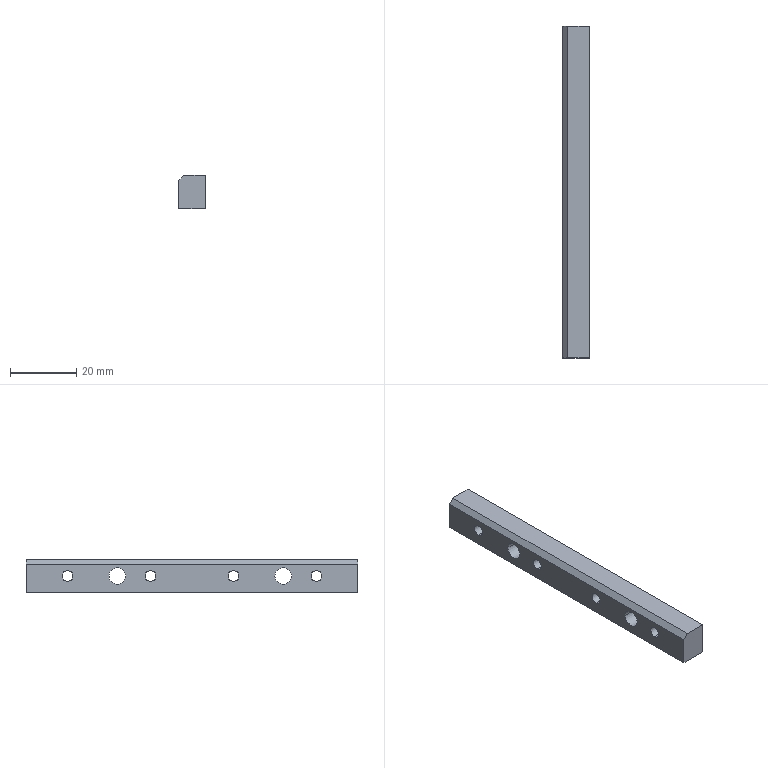Part | NX | 1 solid | 27 faces | box 8 x 100 x 10 mm | volume 7294 mm3 | cylinder 12 | cone 8 | plane 7 | commonest cylinder face diameters 3.3 x8 5 x4
STEP:
#1=CARTESIAN_POINT('',(8.,0.,0.));
#2=VERTEX_POINT('',#1);
#3=CARTESIAN_POINT('',(1.5,0.,0.));
#4=VERTEX_POINT('',#3);
#5=CARTESIAN_POINT('',(8.,0.,0.));
#6=DIRECTION('',(-1.,0.,0.));
#7=VECTOR('',#6,1000.);
#8=LINE('',#5,#7);
#9=EDGE_CURVE('',#2,#4,#8,.T.);
#10=ORIENTED_EDGE('',*,*,#9,.T.);
#11=CARTESIAN_POINT('',(0.,0.,-1.5));
#12=VERTEX_POINT('',#11);
#13=CARTESIAN_POINT('',(0.,0.,-1.5));
#14=DIRECTION('',(0.7071,0.,0.7071));
#15=VECTOR('',#14,1000.);
#16=LINE('',#13,#15);
#17=EDGE_CURVE('',#12,#4,#16,.T.);
#18=ORIENTED_EDGE('',*,*,#17,.F.);
#19=CARTESIAN_POINT('',(0.,0.,-10.));
#20=VERTEX_POINT('',#19);
#21=CARTESIAN_POINT('',(0.,0.,0.));
#22=DIRECTION('',(0.,0.,1.));
#23=VECTOR('',#22,1000.);
#24=LINE('',#21,#23);
#25=EDGE_CURVE('',#20,#12,#24,.T.);
#26=ORIENTED_EDGE('',*,*,#25,.F.);
#27=CARTESIAN_POINT('',(8.,0.,-10.));
#28=VERTEX_POINT('',#27);
#29=CARTESIAN_POINT('',(0.,0.,-10.));
#30=DIRECTION('',(1.,0.,0.));
#31=VECTOR('',#30,1000.);
#32=LINE('',#29,#31);
#33=EDGE_CURVE('',#20,#28,#32,.T.);
#34=ORIENTED_EDGE('',*,*,#33,.T.);
#35=CARTESIAN_POINT('',(8.,0.,0.));
#36=DIRECTION('',(0.,0.,-1.));
#37=VECTOR('',#36,1000.);
#38=LINE('',#35,#37);
#39=EDGE_CURVE('',#2,#28,#38,.T.);
#40=ORIENTED_EDGE('',*,*,#39,.F.);
#41=EDGE_LOOP('',(#10,#18,#26,#34,#40));
#42=FACE_BOUND('',#41,.T.);
#43=CARTESIAN_POINT('',(0.,0.,0.));
#44=DIRECTION('',(0.,1.,0.));
#45=DIRECTION('',(1.,0.,0.));
#46=AXIS2_PLACEMENT_3D('',#43,#44,#45);
#47=PLANE('',#46);
#48=ADVANCED_FACE('',(#42),#47,.F.);
#49=ORIENTED_EDGE('',*,*,#9,.F.);
#50=CARTESIAN_POINT('',(8.,100.,0.));
#51=VERTEX_POINT('',#50);
#52=CARTESIAN_POINT('',(8.,0.,0.));
#53=DIRECTION('',(0.,1.,0.));
#54=VECTOR('',#53,1000.);
#55=LINE('',#52,#54);
#56=EDGE_CURVE('',#2,#51,#55,.T.);
#57=ORIENTED_EDGE('',*,*,#56,.T.);
#58=CARTESIAN_POINT('',(1.5,100.,0.));
#59=VERTEX_POINT('',#58);
#60=CARTESIAN_POINT('',(8.,100.,0.));
#61=DIRECTION('',(-1.,0.,0.));
#62=VECTOR('',#61,1000.);
#63=LINE('',#60,#62);
#64=EDGE_CURVE('',#51,#59,#63,.T.);
#65=ORIENTED_EDGE('',*,*,#64,.T.);
#66=CARTESIAN_POINT('',(1.5,100.,0.));
#67=DIRECTION('',(0.,-1.,0.));
#68=VECTOR('',#67,1000.);
#69=LINE('',#66,#68);
#70=EDGE_CURVE('',#59,#4,#69,.T.);
#71=ORIENTED_EDGE('',*,*,#70,.T.);
#72=EDGE_LOOP('',(#49,#57,#65,#71));
#73=FACE_BOUND('',#72,.T.);
#74=CARTESIAN_POINT('',(0.,0.,0.));
#75=DIRECTION('',(0.,0.,1.));
#76=DIRECTION('',(1.,0.,0.));
#77=AXIS2_PLACEMENT_3D('',#74,#75,#76);
#78=PLANE('',#77);
#79=ADVANCED_FACE('',(#73),#78,.T.);
#80=ORIENTED_EDGE('',*,*,#70,.F.);
#81=CARTESIAN_POINT('',(0.,100.,-1.5));
#82=VERTEX_POINT('',#81);
#83=CARTESIAN_POINT('',(1.5,100.,0.));
#84=DIRECTION('',(-0.7071,0.,-0.7071));
#85=VECTOR('',#84,1000.);
#86=LINE('',#83,#85);
#87=EDGE_CURVE('',#59,#82,#86,.T.);
#88=ORIENTED_EDGE('',*,*,#87,.T.);
#89=CARTESIAN_POINT('',(0.,0.,-1.5));
#90=DIRECTION('',(0.,-1.,0.));
#91=VECTOR('',#90,1000.);
#92=LINE('',#89,#91);
#93=EDGE_CURVE('',#82,#12,#92,.T.);
#94=ORIENTED_EDGE('',*,*,#93,.T.);
#95=ORIENTED_EDGE('',*,*,#17,.T.);
#96=EDGE_LOOP('',(#80,#88,#94,#95));
#97=FACE_BOUND('',#96,.T.);
#98=CARTESIAN_POINT('',(1.5,0.,0.));
#99=DIRECTION('',(-0.7071,0.,0.7071));
#100=DIRECTION('',(0.,1.,0.));
#101=AXIS2_PLACEMENT_3D('',#98,#99,#100);
#102=PLANE('',#101);
#103=ADVANCED_FACE('',(#97),#102,.T.);
#104=ORIENTED_EDGE('',*,*,#39,.T.);
#105=CARTESIAN_POINT('',(8.,100.,-10.));
#106=VERTEX_POINT('',#105);
#107=CARTESIAN_POINT('',(8.,0.,-10.));
#108=DIRECTION('',(0.,-1.,0.));
#109=VECTOR('',#108,1000.);
#110=LINE('',#107,#109);
#111=EDGE_CURVE('',#106,#28,#110,.T.);
#112=ORIENTED_EDGE('',*,*,#111,.F.);
#113=CARTESIAN_POINT('',(8.,100.,0.));
#114=DIRECTION('',(0.,0.,-1.));
#115=VECTOR('',#114,1000.);
#116=LINE('',#113,#115);
#117=EDGE_CURVE('',#51,#106,#116,.T.);
#118=ORIENTED_EDGE('',*,*,#117,.F.);
#119=ORIENTED_EDGE('',*,*,#56,.F.);
#120=EDGE_LOOP('',(#104,#112,#118,#119));
#121=FACE_BOUND('',#120,.T.);
#122=CARTESIAN_POINT('',(8.,20.,-5.));
#123=VERTEX_POINT('',#122);
#124=CARTESIAN_POINT('',(8.,25.,-5.));
#125=VERTEX_POINT('',#124);
#126=CARTESIAN_POINT('',(8.,22.5,-5.));
#127=DIRECTION('',(1.,0.,0.));
#128=DIRECTION('',(0.,1.,0.));
#129=AXIS2_PLACEMENT_3D('',#126,#127,#128);
#130=CIRCLE('',#129,2.5);
#131=EDGE_CURVE('',#123,#125,#130,.T.);
#132=ORIENTED_EDGE('',*,*,#131,.F.);
#133=CARTESIAN_POINT('',(8.,22.5,-5.));
#134=DIRECTION('',(1.,0.,0.));
#135=DIRECTION('',(0.,1.,0.));
#136=AXIS2_PLACEMENT_3D('',#133,#134,#135);
#137=CIRCLE('',#136,2.5);
#138=EDGE_CURVE('',#125,#123,#137,.T.);
#139=ORIENTED_EDGE('',*,*,#138,.F.);
#140=EDGE_LOOP('',(#132,#139));
#141=FACE_BOUND('',#140,.T.);
#142=CARTESIAN_POINT('',(8.,89.815,-5.));
#143=VERTEX_POINT('',#142);
#144=CARTESIAN_POINT('',(8.,85.185,-5.));
#145=VERTEX_POINT('',#144);
#146=CARTESIAN_POINT('',(8.,87.5,-5.));
#147=DIRECTION('',(1.,0.,0.));
#148=DIRECTION('',(0.,-1.,0.));
#149=AXIS2_PLACEMENT_3D('',#146,#147,#148);
#150=CIRCLE('',#149,2.315);
#151=EDGE_CURVE('',#143,#145,#150,.T.);
#152=ORIENTED_EDGE('',*,*,#151,.F.);
#153=CARTESIAN_POINT('',(8.,87.5,-5.));
#154=DIRECTION('',(1.,0.,0.));
#155=DIRECTION('',(0.,-1.,0.));
#156=AXIS2_PLACEMENT_3D('',#153,#154,#155);
#157=CIRCLE('',#156,2.315);
#158=EDGE_CURVE('',#145,#143,#157,.T.);
#159=ORIENTED_EDGE('',*,*,#158,.F.);
#160=EDGE_LOOP('',(#152,#159));
#161=FACE_BOUND('',#160,.T.);
#162=CARTESIAN_POINT('',(8.,35.185,-5.));
#163=VERTEX_POINT('',#162);
#164=CARTESIAN_POINT('',(8.,39.815,-5.));
#165=VERTEX_POINT('',#164);
#166=CARTESIAN_POINT('',(8.,37.5,-5.));
#167=DIRECTION('',(1.,0.,0.));
#168=DIRECTION('',(0.,-1.,0.));
#169=AXIS2_PLACEMENT_3D('',#166,#167,#168);
#170=CIRCLE('',#169,2.315);
#171=EDGE_CURVE('',#163,#165,#170,.T.);
#172=ORIENTED_EDGE('',*,*,#171,.F.);
#173=CARTESIAN_POINT('',(8.,37.5,-5.));
#174=DIRECTION('',(1.,0.,0.));
#175=DIRECTION('',(0.,-1.,0.));
#176=AXIS2_PLACEMENT_3D('',#173,#174,#175);
#177=CIRCLE('',#176,2.315);
#178=EDGE_CURVE('',#165,#163,#177,.T.);
#179=ORIENTED_EDGE('',*,*,#178,.F.);
#180=EDGE_LOOP('',(#172,#179));
#181=FACE_BOUND('',#180,.T.);
#182=CARTESIAN_POINT('',(8.,70.,-5.));
#183=VERTEX_POINT('',#182);
#184=CARTESIAN_POINT('',(8.,75.,-5.));
#185=VERTEX_POINT('',#184);
#186=CARTESIAN_POINT('',(8.,72.5,-5.));
#187=DIRECTION('',(1.,0.,0.));
#188=DIRECTION('',(0.,1.,0.));
#189=AXIS2_PLACEMENT_3D('',#186,#187,#188);
#190=CIRCLE('',#189,2.5);
#191=EDGE_CURVE('',#183,#185,#190,.T.);
#192=ORIENTED_EDGE('',*,*,#191,.F.);
#193=CARTESIAN_POINT('',(8.,72.5,-5.));
#194=DIRECTION('',(1.,0.,0.));
#195=DIRECTION('',(0.,1.,0.));
#196=AXIS2_PLACEMENT_3D('',#193,#194,#195);
#197=CIRCLE('',#196,2.5);
#198=EDGE_CURVE('',#185,#183,#197,.T.);
#199=ORIENTED_EDGE('',*,*,#198,.F.);
#200=EDGE_LOOP('',(#192,#199));
#201=FACE_BOUND('',#200,.T.);
#202=CARTESIAN_POINT('',(8.,10.185,-5.));
#203=VERTEX_POINT('',#202);
#204=CARTESIAN_POINT('',(8.,14.815,-5.));
#205=VERTEX_POINT('',#204);
#206=CARTESIAN_POINT('',(8.,12.5,-5.));
#207=DIRECTION('',(1.,0.,0.));
#208=DIRECTION('',(0.,-1.,0.));
#209=AXIS2_PLACEMENT_3D('',#206,#207,#208);
#210=CIRCLE('',#209,2.315);
#211=EDGE_CURVE('',#203,#205,#210,.T.);
#212=ORIENTED_EDGE('',*,*,#211,.F.);
#213=CARTESIAN_POINT('',(8.,12.5,-5.));
#214=DIRECTION('',(1.,0.,0.));
#215=DIRECTION('',(0.,-1.,0.));
#216=AXIS2_PLACEMENT_3D('',#213,#214,#215);
#217=CIRCLE('',#216,2.315);
#218=EDGE_CURVE('',#205,#203,#217,.T.);
#219=ORIENTED_EDGE('',*,*,#218,.F.);
#220=EDGE_LOOP('',(#212,#219));
#221=FACE_BOUND('',#220,.T.);
#222=CARTESIAN_POINT('',(8.,64.815,-5.));
#223=VERTEX_POINT('',#222);
#224=CARTESIAN_POINT('',(8.,60.185,-5.));
#225=VERTEX_POINT('',#224);
#226=CARTESIAN_POINT('',(8.,62.5,-5.));
#227=DIRECTION('',(1.,0.,0.));
#228=DIRECTION('',(0.,-1.,0.));
#229=AXIS2_PLACEMENT_3D('',#226,#227,#228);
#230=CIRCLE('',#229,2.315);
#231=EDGE_CURVE('',#223,#225,#230,.T.);
#232=ORIENTED_EDGE('',*,*,#231,.F.);
#233=CARTESIAN_POINT('',(8.,62.5,-5.));
#234=DIRECTION('',(1.,0.,0.));
#235=DIRECTION('',(0.,-1.,0.));
#236=AXIS2_PLACEMENT_3D('',#233,#234,#235);
#237=CIRCLE('',#236,2.315);
#238=EDGE_CURVE('',#225,#223,#237,.T.);
#239=ORIENTED_EDGE('',*,*,#238,.F.);
#240=EDGE_LOOP('',(#232,#239));
#241=FACE_BOUND('',#240,.T.);
#242=CARTESIAN_POINT('',(8.,0.,0.));
#243=DIRECTION('',(1.,0.,0.));
#244=DIRECTION('',(0.,1.,0.));
#245=AXIS2_PLACEMENT_3D('',#242,#243,#244);
#246=PLANE('',#245);
#247=ADVANCED_FACE('',(#121,#141,#161,#181,#201,#221,#241),#246,.T.);
#248=ORIENTED_EDGE('',*,*,#33,.F.);
#249=CARTESIAN_POINT('',(0.,100.,-10.));
#250=VERTEX_POINT('',#249);
#251=CARTESIAN_POINT('',(0.,0.,-10.));
#252=DIRECTION('',(0.,1.,0.));
#253=VECTOR('',#252,1000.);
#254=LINE('',#251,#253);
#255=EDGE_CURVE('',#20,#250,#254,.T.);
#256=ORIENTED_EDGE('',*,*,#255,.T.);
#257=CARTESIAN_POINT('',(0.,100.,-10.));
#258=DIRECTION('',(1.,0.,0.));
#259=VECTOR('',#258,1000.);
#260=LINE('',#257,#259);
#261=EDGE_CURVE('',#250,#106,#260,.T.);
#262=ORIENTED_EDGE('',*,*,#261,.T.);
#263=ORIENTED_EDGE('',*,*,#111,.T.);
#264=EDGE_LOOP('',(#248,#256,#262,#263));
#265=FACE_BOUND('',#264,.T.);
#266=CARTESIAN_POINT('',(8.,0.,-10.));
#267=DIRECTION('',(0.,0.,-1.));
#268=DIRECTION('',(0.,-1.,0.));
#269=AXIS2_PLACEMENT_3D('',#266,#267,#268);
#270=PLANE('',#269);
#271=ADVANCED_FACE('',(#265),#270,.T.);
#272=ORIENTED_EDGE('',*,*,#25,.T.);
#273=ORIENTED_EDGE('',*,*,#93,.F.);
#274=CARTESIAN_POINT('',(0.,100.,0.));
#275=DIRECTION('',(0.,0.,1.));
#276=VECTOR('',#275,1000.);
#277=LINE('',#274,#276);
#278=EDGE_CURVE('',#250,#82,#277,.T.);
#279=ORIENTED_EDGE('',*,*,#278,.F.);
#280=ORIENTED_EDGE('',*,*,#255,.F.);
#281=EDGE_LOOP('',(#272,#273,#279,#280));
#282=FACE_BOUND('',#281,.T.);
#283=CARTESIAN_POINT('',(0.,20.,-5.));
#284=VERTEX_POINT('',#283);
#285=CARTESIAN_POINT('',(0.,25.,-5.));
#286=VERTEX_POINT('',#285);
#287=CARTESIAN_POINT('',(0.,22.5,-5.));
#288=DIRECTION('',(1.,0.,0.));
#289=DIRECTION('',(0.,1.,0.));
#290=AXIS2_PLACEMENT_3D('',#287,#288,#289);
#291=CIRCLE('',#290,2.5);
#292=EDGE_CURVE('',#284,#286,#291,.T.);
#293=ORIENTED_EDGE('',*,*,#292,.T.);
#294=CARTESIAN_POINT('',(0.,22.5,-5.));
#295=DIRECTION('',(1.,0.,0.));
#296=DIRECTION('',(0.,1.,0.));
#297=AXIS2_PLACEMENT_3D('',#294,#295,#296);
#298=CIRCLE('',#297,2.5);
#299=EDGE_CURVE('',#286,#284,#298,.T.);
#300=ORIENTED_EDGE('',*,*,#299,.T.);
#301=EDGE_LOOP('',(#293,#300));
#302=FACE_BOUND('',#301,.T.);
#303=CARTESIAN_POINT('',(0.,75.,-5.));
#304=VERTEX_POINT('',#303);
#305=CARTESIAN_POINT('',(0.,70.,-5.));
#306=VERTEX_POINT('',#305);
#307=CARTESIAN_POINT('',(0.,72.5,-5.));
#308=DIRECTION('',(1.,0.,0.));
#309=DIRECTION('',(0.,1.,0.));
#310=AXIS2_PLACEMENT_3D('',#307,#308,#309);
#311=CIRCLE('',#310,2.5);
#312=EDGE_CURVE('',#304,#306,#311,.T.);
#313=ORIENTED_EDGE('',*,*,#312,.T.);
#314=CARTESIAN_POINT('',(0.,72.5,-5.));
#315=DIRECTION('',(1.,0.,0.));
#316=DIRECTION('',(0.,1.,0.));
#317=AXIS2_PLACEMENT_3D('',#314,#315,#316);
#318=CIRCLE('',#317,2.5);
#319=EDGE_CURVE('',#306,#304,#318,.T.);
#320=ORIENTED_EDGE('',*,*,#319,.T.);
#321=EDGE_LOOP('',(#313,#320));
#322=FACE_BOUND('',#321,.T.);
#323=CARTESIAN_POINT('',(0.,12.5,-6.65));
#324=VERTEX_POINT('',#323);
#325=CARTESIAN_POINT('',(0.,12.5,-3.35));
#326=VERTEX_POINT('',#325);
#327=CARTESIAN_POINT('',(0.,12.5,-5.));
#328=DIRECTION('',(1.,0.,0.));
#329=DIRECTION('',(0.,0.,1.));
#330=AXIS2_PLACEMENT_3D('',#327,#328,#329);
#331=CIRCLE('',#330,1.65);
#332=EDGE_CURVE('',#324,#326,#331,.T.);
#333=ORIENTED_EDGE('',*,*,#332,.T.);
#334=CARTESIAN_POINT('',(0.,12.5,-5.));
#335=DIRECTION('',(1.,0.,0.));
#336=DIRECTION('',(0.,0.,1.));
#337=AXIS2_PLACEMENT_3D('',#334,#335,#336);
#338=CIRCLE('',#337,1.65);
#339=EDGE_CURVE('',#326,#324,#338,.T.);
#340=ORIENTED_EDGE('',*,*,#339,.T.);
#341=EDGE_LOOP('',(#333,#340));
#342=FACE_BOUND('',#341,.T.);
#343=CARTESIAN_POINT('',(0.,37.5,-3.35));
#344=VERTEX_POINT('',#343);
#345=CARTESIAN_POINT('',(0.,37.5,-6.65));
#346=VERTEX_POINT('',#345);
#347=CARTESIAN_POINT('',(0.,37.5,-5.));
#348=DIRECTION('',(1.,0.,0.));
#349=DIRECTION('',(0.,0.,1.));
#350=AXIS2_PLACEMENT_3D('',#347,#348,#349);
#351=CIRCLE('',#350,1.65);
#352=EDGE_CURVE('',#344,#346,#351,.T.);
#353=ORIENTED_EDGE('',*,*,#352,.T.);
#354=CARTESIAN_POINT('',(0.,37.5,-5.));
#355=DIRECTION('',(1.,0.,0.));
#356=DIRECTION('',(0.,0.,1.));
#357=AXIS2_PLACEMENT_3D('',#354,#355,#356);
#358=CIRCLE('',#357,1.65);
#359=EDGE_CURVE('',#346,#344,#358,.T.);
#360=ORIENTED_EDGE('',*,*,#359,.T.);
#361=EDGE_LOOP('',(#353,#360));
#362=FACE_BOUND('',#361,.T.);
#363=CARTESIAN_POINT('',(0.,62.5,-3.35));
#364=VERTEX_POINT('',#363);
#365=CARTESIAN_POINT('',(0.,62.5,-6.65));
#366=VERTEX_POINT('',#365);
#367=CARTESIAN_POINT('',(0.,62.5,-5.));
#368=DIRECTION('',(1.,0.,0.));
#369=DIRECTION('',(0.,0.,1.));
#370=AXIS2_PLACEMENT_3D('',#367,#368,#369);
#371=CIRCLE('',#370,1.65);
#372=EDGE_CURVE('',#364,#366,#371,.T.);
#373=ORIENTED_EDGE('',*,*,#372,.T.);
#374=CARTESIAN_POINT('',(0.,62.5,-5.));
#375=DIRECTION('',(1.,0.,0.));
#376=DIRECTION('',(0.,0.,1.));
#377=AXIS2_PLACEMENT_3D('',#374,#375,#376);
#378=CIRCLE('',#377,1.65);
#379=EDGE_CURVE('',#366,#364,#378,.T.);
#380=ORIENTED_EDGE('',*,*,#379,.T.);
#381=EDGE_LOOP('',(#373,#380));
#382=FACE_BOUND('',#381,.T.);
#383=CARTESIAN_POINT('',(0.,87.5,-3.35));
#384=VERTEX_POINT('',#383);
#385=CARTESIAN_POINT('',(0.,87.5,-6.65));
#386=VERTEX_POINT('',#385);
#387=CARTESIAN_POINT('',(0.,87.5,-5.));
#388=DIRECTION('',(1.,0.,0.));
#389=DIRECTION('',(0.,0.,1.));
#390=AXIS2_PLACEMENT_3D('',#387,#388,#389);
#391=CIRCLE('',#390,1.65);
#392=EDGE_CURVE('',#384,#386,#391,.T.);
#393=ORIENTED_EDGE('',*,*,#392,.T.);
#394=CARTESIAN_POINT('',(0.,87.5,-5.));
#395=DIRECTION('',(1.,0.,0.));
#396=DIRECTION('',(0.,0.,1.));
#397=AXIS2_PLACEMENT_3D('',#394,#395,#396);
#398=CIRCLE('',#397,1.65);
#399=EDGE_CURVE('',#386,#384,#398,.T.);
#400=ORIENTED_EDGE('',*,*,#399,.T.);
#401=EDGE_LOOP('',(#393,#400));
#402=FACE_BOUND('',#401,.T.);
#403=CARTESIAN_POINT('',(0.,0.,-10.));
#404=DIRECTION('',(-1.,0.,0.));
#405=DIRECTION('',(0.,0.,1.));
#406=AXIS2_PLACEMENT_3D('',#403,#404,#405);
#407=PLANE('',#406);
#408=ADVANCED_FACE('',(#282,#302,#322,#342,#362,#382,#402),#407,.T.);
#409=ORIENTED_EDGE('',*,*,#64,.F.);
#410=ORIENTED_EDGE('',*,*,#117,.T.);
#411=ORIENTED_EDGE('',*,*,#261,.F.);
#412=ORIENTED_EDGE('',*,*,#278,.T.);
#413=ORIENTED_EDGE('',*,*,#87,.F.);
#414=EDGE_LOOP('',(#409,#410,#411,#412,#413));
#415=FACE_BOUND('',#414,.T.);
#416=CARTESIAN_POINT('',(0.,100.,0.));
#417=DIRECTION('',(0.,1.,0.));
#418=DIRECTION('',(1.,0.,0.));
#419=AXIS2_PLACEMENT_3D('',#416,#417,#418);
#420=PLANE('',#419);
#421=ADVANCED_FACE('',(#415),#420,.T.);
#422=ORIENTED_EDGE('',*,*,#131,.T.);
#423=CARTESIAN_POINT('',(0.,25.,-5.));
#424=DIRECTION('',(1.,0.,0.));
#425=VECTOR('',#424,1000.);
#426=LINE('',#423,#425);
#427=EDGE_CURVE('',#286,#125,#426,.T.);
#428=ORIENTED_EDGE('',*,*,#427,.F.);
#429=ORIENTED_EDGE('',*,*,#292,.F.);
#430=CARTESIAN_POINT('',(0.,20.,-5.));
#431=DIRECTION('',(1.,0.,0.));
#432=VECTOR('',#431,1000.);
#433=LINE('',#430,#432);
#434=EDGE_CURVE('',#284,#123,#433,.T.);
#435=ORIENTED_EDGE('',*,*,#434,.T.);
#436=EDGE_LOOP('',(#422,#428,#429,#435));
#437=FACE_BOUND('',#436,.T.);
#438=CARTESIAN_POINT('',(0.,22.5,-5.));
#439=DIRECTION('',(1.,0.,0.));
#440=DIRECTION('',(0.,1.,0.));
#441=AXIS2_PLACEMENT_3D('',#438,#439,#440);
#442=CYLINDRICAL_SURFACE('',#441,2.5);
#443=ADVANCED_FACE('',(#437),#442,.F.);
#444=ORIENTED_EDGE('',*,*,#312,.F.);
#445=CARTESIAN_POINT('',(0.,75.,-5.));
#446=DIRECTION('',(1.,0.,0.));
#447=VECTOR('',#446,1000.);
#448=LINE('',#445,#447);
#449=EDGE_CURVE('',#304,#185,#448,.T.);
#450=ORIENTED_EDGE('',*,*,#449,.T.);
#451=ORIENTED_EDGE('',*,*,#198,.T.);
#452=CARTESIAN_POINT('',(0.,70.,-5.));
#453=DIRECTION('',(1.,0.,0.));
#454=VECTOR('',#453,1000.);
#455=LINE('',#452,#454);
#456=EDGE_CURVE('',#306,#183,#455,.T.);
#457=ORIENTED_EDGE('',*,*,#456,.F.);
#458=EDGE_LOOP('',(#444,#450,#451,#457));
#459=FACE_BOUND('',#458,.T.);
#460=CARTESIAN_POINT('',(0.,72.5,-5.));
#461=DIRECTION('',(1.,0.,0.));
#462=DIRECTION('',(0.,1.,0.));
#463=AXIS2_PLACEMENT_3D('',#460,#461,#462);
#464=CYLINDRICAL_SURFACE('',#463,2.5);
#465=ADVANCED_FACE('',(#459),#464,.F.);
#466=ORIENTED_EDGE('',*,*,#332,.F.);
#467=CARTESIAN_POINT('',(7.616,12.5,-6.65));
#468=VERTEX_POINT('',#467);
#469=CARTESIAN_POINT('',(4.,12.5,-6.65));
#470=DIRECTION('',(1.,0.,0.));
#471=VECTOR('',#470,1000.);
#472=LINE('',#469,#471);
#473=EDGE_CURVE('',#468,#324,#472,.F.);
#474=ORIENTED_EDGE('',*,*,#473,.F.);
#475=CARTESIAN_POINT('',(7.616,14.15,-5.));
#476=VERTEX_POINT('',#475);
#477=CARTESIAN_POINT('',(7.616,12.5,-5.));
#478=DIRECTION('',(1.,0.,0.));
#479=DIRECTION('',(0.,-1.,0.));
#480=AXIS2_PLACEMENT_3D('',#477,#478,#479);
#481=CIRCLE('',#480,1.65);
#482=EDGE_CURVE('',#468,#476,#481,.T.);
#483=ORIENTED_EDGE('',*,*,#482,.T.);
#484=CARTESIAN_POINT('',(7.616,12.5,-3.35));
#485=VERTEX_POINT('',#484);
#486=CARTESIAN_POINT('',(7.616,12.5,-5.));
#487=DIRECTION('',(1.,0.,0.));
#488=DIRECTION('',(0.,-1.,0.));
#489=AXIS2_PLACEMENT_3D('',#486,#487,#488);
#490=CIRCLE('',#489,1.65);
#491=EDGE_CURVE('',#476,#485,#490,.T.);
#492=ORIENTED_EDGE('',*,*,#491,.T.);
#493=CARTESIAN_POINT('',(4.,12.5,-3.35));
#494=DIRECTION('',(1.,0.,0.));
#495=VECTOR('',#494,1000.);
#496=LINE('',#493,#495);
#497=EDGE_CURVE('',#485,#326,#496,.F.);
#498=ORIENTED_EDGE('',*,*,#497,.T.);
#499=EDGE_LOOP('',(#466,#474,#483,#492,#498));
#500=FACE_BOUND('',#499,.T.);
#501=CARTESIAN_POINT('',(4.,12.5,-5.));
#502=DIRECTION('',(1.,0.,0.));
#503=DIRECTION('',(0.,0.,1.));
#504=AXIS2_PLACEMENT_3D('',#501,#502,#503);
#505=CYLINDRICAL_SURFACE('',#504,1.65);
#506=ADVANCED_FACE('',(#500),#505,.F.);
#507=ORIENTED_EDGE('',*,*,#211,.T.);
#508=CARTESIAN_POINT('',(7.616,14.15,-5.));
#509=DIRECTION('',(0.5,0.866,0.));
#510=VECTOR('',#509,1000.);
#511=LINE('',#508,#510);
#512=EDGE_CURVE('',#205,#476,#511,.F.);
#513=ORIENTED_EDGE('',*,*,#512,.T.);
#514=ORIENTED_EDGE('',*,*,#482,.F.);
#515=CARTESIAN_POINT('',(7.616,10.85,-5.));
#516=VERTEX_POINT('',#515);
#517=CARTESIAN_POINT('',(7.616,12.5,-5.));
#518=DIRECTION('',(1.,0.,0.));
#519=DIRECTION('',(0.,-1.,0.));
#520=AXIS2_PLACEMENT_3D('',#517,#518,#519);
#521=CIRCLE('',#520,1.65);
#522=EDGE_CURVE('',#516,#468,#521,.T.);
#523=ORIENTED_EDGE('',*,*,#522,.F.);
#524=CARTESIAN_POINT('',(7.616,10.85,-5.));
#525=DIRECTION('',(0.5,-0.866,0.));
#526=VECTOR('',#525,1000.);
#527=LINE('',#524,#526);
#528=EDGE_CURVE('',#203,#516,#527,.F.);
#529=ORIENTED_EDGE('',*,*,#528,.F.);
#530=EDGE_LOOP('',(#507,#513,#514,#523,#529));
#531=FACE_BOUND('',#530,.T.);
#532=CARTESIAN_POINT('',(7.616,12.5,-5.));
#533=DIRECTION('',(1.,0.,0.));
#534=DIRECTION('',(0.,-1.,0.));
#535=AXIS2_PLACEMENT_3D('',#532,#533,#534);
#536=CONICAL_SURFACE('',#535,1.65,1.047);
#537=ADVANCED_FACE('',(#531),#536,.F.);
#538=ORIENTED_EDGE('',*,*,#352,.F.);
#539=CARTESIAN_POINT('',(7.616,37.5,-3.35));
#540=VERTEX_POINT('',#539);
#541=CARTESIAN_POINT('',(4.,37.5,-3.35));
#542=DIRECTION('',(1.,0.,0.));
#543=VECTOR('',#542,1000.);
#544=LINE('',#541,#543);
#545=EDGE_CURVE('',#344,#540,#544,.T.);
#546=ORIENTED_EDGE('',*,*,#545,.T.);
#547=CARTESIAN_POINT('',(7.616,35.85,-5.));
#548=VERTEX_POINT('',#547);
#549=CARTESIAN_POINT('',(7.616,37.5,-5.));
#550=DIRECTION('',(1.,0.,0.));
#551=DIRECTION('',(0.,-1.,0.));
#552=AXIS2_PLACEMENT_3D('',#549,#550,#551);
#553=CIRCLE('',#552,1.65);
#554=EDGE_CURVE('',#540,#548,#553,.T.);
#555=ORIENTED_EDGE('',*,*,#554,.T.);
#556=CARTESIAN_POINT('',(7.616,37.5,-6.65));
#557=VERTEX_POINT('',#556);
#558=CARTESIAN_POINT('',(7.616,37.5,-5.));
#559=DIRECTION('',(1.,0.,0.));
#560=DIRECTION('',(0.,-1.,0.));
#561=AXIS2_PLACEMENT_3D('',#558,#559,#560);
#562=CIRCLE('',#561,1.65);
#563=EDGE_CURVE('',#548,#557,#562,.T.);
#564=ORIENTED_EDGE('',*,*,#563,.T.);
#565=CARTESIAN_POINT('',(4.,37.5,-6.65));
#566=DIRECTION('',(1.,0.,0.));
#567=VECTOR('',#566,1000.);
#568=LINE('',#565,#567);
#569=EDGE_CURVE('',#346,#557,#568,.T.);
#570=ORIENTED_EDGE('',*,*,#569,.F.);
#571=EDGE_LOOP('',(#538,#546,#555,#564,#570));
#572=FACE_BOUND('',#571,.T.);
#573=CARTESIAN_POINT('',(4.,37.5,-5.));
#574=DIRECTION('',(1.,0.,0.));
#575=DIRECTION('',(0.,0.,1.));
#576=AXIS2_PLACEMENT_3D('',#573,#574,#575);
#577=CYLINDRICAL_SURFACE('',#576,1.65);
#578=ADVANCED_FACE('',(#572),#577,.F.);
#579=CARTESIAN_POINT('',(7.616,39.15,-5.));
#580=VERTEX_POINT('',#579);
#581=CARTESIAN_POINT('',(7.616,37.5,-5.));
#582=DIRECTION('',(1.,0.,0.));
#583=DIRECTION('',(0.,-1.,0.));
#584=AXIS2_PLACEMENT_3D('',#581,#582,#583);
#585=CIRCLE('',#584,1.65);
#586=EDGE_CURVE('',#557,#580,#585,.T.);
#587=ORIENTED_EDGE('',*,*,#586,.F.);
#588=ORIENTED_EDGE('',*,*,#563,.F.);
#589=CARTESIAN_POINT('',(7.616,35.85,-5.));
#590=DIRECTION('',(0.5,-0.866,0.));
#591=VECTOR('',#590,1000.);
#592=LINE('',#589,#591);
#593=EDGE_CURVE('',#163,#548,#592,.F.);
#594=ORIENTED_EDGE('',*,*,#593,.F.);
#595=ORIENTED_EDGE('',*,*,#171,.T.);
#596=CARTESIAN_POINT('',(7.616,39.15,-5.));
#597=DIRECTION('',(0.5,0.866,0.));
#598=VECTOR('',#597,1000.);
#599=LINE('',#596,#598);
#600=EDGE_CURVE('',#165,#580,#599,.F.);
#601=ORIENTED_EDGE('',*,*,#600,.T.);
#602=EDGE_LOOP('',(#587,#588,#594,#595,#601));
#603=FACE_BOUND('',#602,.T.);
#604=CARTESIAN_POINT('',(7.616,37.5,-5.));
#605=DIRECTION('',(1.,0.,0.));
#606=DIRECTION('',(0.,-1.,0.));
#607=AXIS2_PLACEMENT_3D('',#604,#605,#606);
#608=CONICAL_SURFACE('',#607,1.65,1.047);
#609=ADVANCED_FACE('',(#603),#608,.F.);
#610=CARTESIAN_POINT('',(7.616,62.5,-6.65));
#611=VERTEX_POINT('',#610);
#612=CARTESIAN_POINT('',(7.616,64.15,-5.));
#613=VERTEX_POINT('',#612);
#614=CARTESIAN_POINT('',(7.616,62.5,-5.));
#615=DIRECTION('',(1.,0.,0.));
#616=DIRECTION('',(0.,-1.,0.));
#617=AXIS2_PLACEMENT_3D('',#614,#615,#616);
#618=CIRCLE('',#617,1.65);
#619=EDGE_CURVE('',#611,#613,#618,.T.);
#620=ORIENTED_EDGE('',*,*,#619,.T.);
#621=CARTESIAN_POINT('',(7.616,62.5,-3.35));
#622=VERTEX_POINT('',#621);
#623=CARTESIAN_POINT('',(7.616,62.5,-5.));
#624=DIRECTION('',(1.,0.,0.));
#625=DIRECTION('',(0.,-1.,0.));
#626=AXIS2_PLACEMENT_3D('',#623,#624,#625);
#627=CIRCLE('',#626,1.65);
#628=EDGE_CURVE('',#613,#622,#627,.T.);
#629=ORIENTED_EDGE('',*,*,#628,.T.);
#630=CARTESIAN_POINT('',(4.,62.5,-3.35));
#631=DIRECTION('',(1.,0.,0.));
#632=VECTOR('',#631,1000.);
#633=LINE('',#630,#632);
#634=EDGE_CURVE('',#364,#622,#633,.T.);
#635=ORIENTED_EDGE('',*,*,#634,.F.);
#636=ORIENTED_EDGE('',*,*,#379,.F.);
#637=CARTESIAN_POINT('',(4.,62.5,-6.65));
#638=DIRECTION('',(1.,0.,0.));
#639=VECTOR('',#638,1000.);
#640=LINE('',#637,#639);
#641=EDGE_CURVE('',#366,#611,#640,.T.);
#642=ORIENTED_EDGE('',*,*,#641,.T.);
#643=EDGE_LOOP('',(#620,#629,#635,#636,#642));
#644=FACE_BOUND('',#643,.T.);
#645=CARTESIAN_POINT('',(4.,62.5,-5.));
#646=DIRECTION('',(1.,0.,0.));
#647=DIRECTION('',(0.,0.,1.));
#648=AXIS2_PLACEMENT_3D('',#645,#646,#647);
#649=CYLINDRICAL_SURFACE('',#648,1.65);
#650=ADVANCED_FACE('',(#644),#649,.F.);
#651=ORIENTED_EDGE('',*,*,#619,.F.);
#652=CARTESIAN_POINT('',(7.616,60.85,-5.));
#653=VERTEX_POINT('',#652);
#654=CARTESIAN_POINT('',(7.616,62.5,-5.));
#655=DIRECTION('',(1.,0.,0.));
#656=DIRECTION('',(0.,-1.,0.));
#657=AXIS2_PLACEMENT_3D('',#654,#655,#656);
#658=CIRCLE('',#657,1.65);
#659=EDGE_CURVE('',#653,#611,#658,.T.);
#660=ORIENTED_EDGE('',*,*,#659,.F.);
#661=CARTESIAN_POINT('',(7.616,60.85,-5.));
#662=DIRECTION('',(0.5,-0.866,0.));
#663=VECTOR('',#662,1000.);
#664=LINE('',#661,#663);
#665=EDGE_CURVE('',#225,#653,#664,.F.);
#666=ORIENTED_EDGE('',*,*,#665,.F.);
#667=ORIENTED_EDGE('',*,*,#238,.T.);
#668=CARTESIAN_POINT('',(7.616,64.15,-5.));
#669=DIRECTION('',(0.5,0.866,0.));
#670=VECTOR('',#669,1000.);
#671=LINE('',#668,#670);
#672=EDGE_CURVE('',#223,#613,#671,.F.);
#673=ORIENTED_EDGE('',*,*,#672,.T.);
#674=EDGE_LOOP('',(#651,#660,#666,#667,#673));
#675=FACE_BOUND('',#674,.T.);
#676=CARTESIAN_POINT('',(7.616,62.5,-5.));
#677=DIRECTION('',(1.,0.,0.));
#678=DIRECTION('',(0.,-1.,0.));
#679=AXIS2_PLACEMENT_3D('',#676,#677,#678);
#680=CONICAL_SURFACE('',#679,1.65,1.047);
#681=ADVANCED_FACE('',(#675),#680,.F.);
#682=ORIENTED_EDGE('',*,*,#392,.F.);
#683=CARTESIAN_POINT('',(7.616,87.5,-3.35));
#684=VERTEX_POINT('',#683);
#685=CARTESIAN_POINT('',(4.,87.5,-3.35));
#686=DIRECTION('',(1.,0.,0.));
#687=VECTOR('',#686,1000.);
#688=LINE('',#685,#687);
#689=EDGE_CURVE('',#384,#684,#688,.T.);
#690=ORIENTED_EDGE('',*,*,#689,.T.);
#691=CARTESIAN_POINT('',(7.616,85.85,-5.));
#692=VERTEX_POINT('',#691);
#693=CARTESIAN_POINT('',(7.616,87.5,-5.));
#694=DIRECTION('',(1.,0.,0.));
#695=DIRECTION('',(0.,-1.,0.));
#696=AXIS2_PLACEMENT_3D('',#693,#694,#695);
#697=CIRCLE('',#696,1.65);
#698=EDGE_CURVE('',#684,#692,#697,.T.);
#699=ORIENTED_EDGE('',*,*,#698,.T.);
#700=CARTESIAN_POINT('',(7.616,87.5,-6.65));
#701=VERTEX_POINT('',#700);
#702=CARTESIAN_POINT('',(7.616,87.5,-5.));
#703=DIRECTION('',(1.,0.,0.));
#704=DIRECTION('',(0.,-1.,0.));
#705=AXIS2_PLACEMENT_3D('',#702,#703,#704);
#706=CIRCLE('',#705,1.65);
#707=EDGE_CURVE('',#692,#701,#706,.T.);
#708=ORIENTED_EDGE('',*,*,#707,.T.);
#709=CARTESIAN_POINT('',(4.,87.5,-6.65));
#710=DIRECTION('',(1.,0.,0.));
#711=VECTOR('',#710,1000.);
#712=LINE('',#709,#711);
#713=EDGE_CURVE('',#386,#701,#712,.T.);
#714=ORIENTED_EDGE('',*,*,#713,.F.);
#715=EDGE_LOOP('',(#682,#690,#699,#708,#714));
#716=FACE_BOUND('',#715,.T.);
#717=CARTESIAN_POINT('',(4.,87.5,-5.));
#718=DIRECTION('',(1.,0.,0.));
#719=DIRECTION('',(0.,0.,1.));
#720=AXIS2_PLACEMENT_3D('',#717,#718,#719);
#721=CYLINDRICAL_SURFACE('',#720,1.65);
#722=ADVANCED_FACE('',(#716),#721,.F.);
#723=CARTESIAN_POINT('',(7.616,89.15,-5.));
#724=VERTEX_POINT('',#723);
#725=CARTESIAN_POINT('',(7.616,87.5,-5.));
#726=DIRECTION('',(1.,0.,0.));
#727=DIRECTION('',(0.,-1.,0.));
#728=AXIS2_PLACEMENT_3D('',#725,#726,#727);
#729=CIRCLE('',#728,1.65);
#730=EDGE_CURVE('',#701,#724,#729,.T.);
#731=ORIENTED_EDGE('',*,*,#730,.F.);
#732=ORIENTED_EDGE('',*,*,#707,.F.);
#733=CARTESIAN_POINT('',(8.,85.185,-5.));
#734=DIRECTION('',(0.5,-0.866,0.));
#735=VECTOR('',#734,1000.);
#736=LINE('',#733,#735);
#737=EDGE_CURVE('',#145,#692,#736,.F.);
#738=ORIENTED_EDGE('',*,*,#737,.F.);
#739=ORIENTED_EDGE('',*,*,#158,.T.);
#740=CARTESIAN_POINT('',(8.,89.815,-5.));
#741=DIRECTION('',(0.5,0.866,0.));
#742=VECTOR('',#741,1000.);
#743=LINE('',#740,#742);
#744=EDGE_CURVE('',#143,#724,#743,.F.);
#745=ORIENTED_EDGE('',*,*,#744,.T.);
#746=EDGE_LOOP('',(#731,#732,#738,#739,#745));
#747=FACE_BOUND('',#746,.T.);
#748=CARTESIAN_POINT('',(8.,87.5,-5.));
#749=DIRECTION('',(1.,0.,0.));
#750=DIRECTION('',(0.,-1.,0.));
#751=AXIS2_PLACEMENT_3D('',#748,#749,#750);
#752=CONICAL_SURFACE('',#751,2.315,1.047);
#753=ADVANCED_FACE('',(#747),#752,.F.);
#754=ORIENTED_EDGE('',*,*,#231,.T.);
#755=ORIENTED_EDGE('',*,*,#665,.T.);
#756=CARTESIAN_POINT('',(7.616,62.5,-5.));
#757=DIRECTION('',(1.,0.,0.));
#758=DIRECTION('',(0.,-1.,0.));
#759=AXIS2_PLACEMENT_3D('',#756,#757,#758);
#760=CIRCLE('',#759,1.65);
#761=EDGE_CURVE('',#622,#653,#760,.T.);
#762=ORIENTED_EDGE('',*,*,#761,.F.);
#763=ORIENTED_EDGE('',*,*,#628,.F.);
#764=ORIENTED_EDGE('',*,*,#672,.F.);
#765=EDGE_LOOP('',(#754,#755,#762,#763,#764));
#766=FACE_BOUND('',#765,.T.);
#767=CARTESIAN_POINT('',(7.616,62.5,-5.));
#768=DIRECTION('',(1.,0.,0.));
#769=DIRECTION('',(0.,-1.,0.));
#770=AXIS2_PLACEMENT_3D('',#767,#768,#769);
#771=CONICAL_SURFACE('',#770,1.65,1.047);
#772=ADVANCED_FACE('',(#766),#771,.F.);
#773=ORIENTED_EDGE('',*,*,#586,.T.);
#774=CARTESIAN_POINT('',(7.616,37.5,-5.));
#775=DIRECTION('',(1.,0.,0.));
#776=DIRECTION('',(0.,-1.,0.));
#777=AXIS2_PLACEMENT_3D('',#774,#775,#776);
#778=CIRCLE('',#777,1.65);
#779=EDGE_CURVE('',#580,#540,#778,.T.);
#780=ORIENTED_EDGE('',*,*,#779,.T.);
#781=ORIENTED_EDGE('',*,*,#545,.F.);
#782=ORIENTED_EDGE('',*,*,#359,.F.);
#783=ORIENTED_EDGE('',*,*,#569,.T.);
#784=EDGE_LOOP('',(#773,#780,#781,#782,#783));
#785=FACE_BOUND('',#784,.T.);
#786=CARTESIAN_POINT('',(4.,37.5,-5.));
#787=DIRECTION('',(1.,0.,0.));
#788=DIRECTION('',(0.,0.,1.));
#789=AXIS2_PLACEMENT_3D('',#786,#787,#788);
#790=CYLINDRICAL_SURFACE('',#789,1.65);
#791=ADVANCED_FACE('',(#785),#790,.F.);
#792=ORIENTED_EDGE('',*,*,#191,.T.);
#793=ORIENTED_EDGE('',*,*,#449,.F.);
#794=ORIENTED_EDGE('',*,*,#319,.F.);
#795=ORIENTED_EDGE('',*,*,#456,.T.);
#796=EDGE_LOOP('',(#792,#793,#794,#795));
#797=FACE_BOUND('',#796,.T.);
#798=CARTESIAN_POINT('',(0.,72.5,-5.));
#799=DIRECTION('',(1.,0.,0.));
#800=DIRECTION('',(0.,1.,0.));
#801=AXIS2_PLACEMENT_3D('',#798,#799,#800);
#802=CYLINDRICAL_SURFACE('',#801,2.5);
#803=ADVANCED_FACE('',(#797),#802,.F.);
#804=ORIENTED_EDGE('',*,*,#730,.T.);
#805=CARTESIAN_POINT('',(7.616,87.5,-5.));
#806=DIRECTION('',(1.,0.,0.));
#807=DIRECTION('',(0.,-1.,0.));
#808=AXIS2_PLACEMENT_3D('',#805,#806,#807);
#809=CIRCLE('',#808,1.65);
#810=EDGE_CURVE('',#724,#684,#809,.T.);
#811=ORIENTED_EDGE('',*,*,#810,.T.);
#812=ORIENTED_EDGE('',*,*,#689,.F.);
#813=ORIENTED_EDGE('',*,*,#399,.F.);
#814=ORIENTED_EDGE('',*,*,#713,.T.);
#815=EDGE_LOOP('',(#804,#811,#812,#813,#814));
#816=FACE_BOUND('',#815,.T.);
#817=CARTESIAN_POINT('',(4.,87.5,-5.));
#818=DIRECTION('',(1.,0.,0.));
#819=DIRECTION('',(0.,0.,1.));
#820=AXIS2_PLACEMENT_3D('',#817,#818,#819);
#821=CYLINDRICAL_SURFACE('',#820,1.65);
#822=ADVANCED_FACE('',(#816),#821,.F.);
#823=ORIENTED_EDGE('',*,*,#593,.T.);
#824=ORIENTED_EDGE('',*,*,#554,.F.);
#825=ORIENTED_EDGE('',*,*,#779,.F.);
#826=ORIENTED_EDGE('',*,*,#600,.F.);
#827=ORIENTED_EDGE('',*,*,#178,.T.);
#828=EDGE_LOOP('',(#823,#824,#825,#826,#827));
#829=FACE_BOUND('',#828,.T.);
#830=CARTESIAN_POINT('',(7.616,37.5,-5.));
#831=DIRECTION('',(1.,0.,0.));
#832=DIRECTION('',(0.,-1.,0.));
#833=AXIS2_PLACEMENT_3D('',#830,#831,#832);
#834=CONICAL_SURFACE('',#833,1.65,1.047);
#835=ADVANCED_FACE('',(#829),#834,.F.);
#836=ORIENTED_EDGE('',*,*,#522,.T.);
#837=ORIENTED_EDGE('',*,*,#473,.T.);
#838=ORIENTED_EDGE('',*,*,#339,.F.);
#839=ORIENTED_EDGE('',*,*,#497,.F.);
#840=CARTESIAN_POINT('',(7.616,12.5,-5.));
#841=DIRECTION('',(1.,0.,0.));
#842=DIRECTION('',(0.,-1.,0.));
#843=AXIS2_PLACEMENT_3D('',#840,#841,#842);
#844=CIRCLE('',#843,1.65);
#845=EDGE_CURVE('',#485,#516,#844,.T.);
#846=ORIENTED_EDGE('',*,*,#845,.T.);
#847=EDGE_LOOP('',(#836,#837,#838,#839,#846));
#848=FACE_BOUND('',#847,.T.);
#849=CARTESIAN_POINT('',(4.,12.5,-5.));
#850=DIRECTION('',(1.,0.,0.));
#851=DIRECTION('',(0.,0.,1.));
#852=AXIS2_PLACEMENT_3D('',#849,#850,#851);
#853=CYLINDRICAL_SURFACE('',#852,1.65);
#854=ADVANCED_FACE('',(#848),#853,.F.);
#855=ORIENTED_EDGE('',*,*,#151,.T.);
#856=ORIENTED_EDGE('',*,*,#737,.T.);
#857=ORIENTED_EDGE('',*,*,#698,.F.);
#858=ORIENTED_EDGE('',*,*,#810,.F.);
#859=ORIENTED_EDGE('',*,*,#744,.F.);
#860=EDGE_LOOP('',(#855,#856,#857,#858,#859));
#861=FACE_BOUND('',#860,.T.);
#862=CARTESIAN_POINT('',(8.,87.5,-5.));
#863=DIRECTION('',(1.,0.,0.));
#864=DIRECTION('',(0.,-1.,0.));
#865=AXIS2_PLACEMENT_3D('',#862,#863,#864);
#866=CONICAL_SURFACE('',#865,2.315,1.047);
#867=ADVANCED_FACE('',(#861),#866,.F.);
#868=ORIENTED_EDGE('',*,*,#372,.F.);
#869=ORIENTED_EDGE('',*,*,#634,.T.);
#870=ORIENTED_EDGE('',*,*,#761,.T.);
#871=ORIENTED_EDGE('',*,*,#659,.T.);
#872=ORIENTED_EDGE('',*,*,#641,.F.);
#873=EDGE_LOOP('',(#868,#869,#870,#871,#872));
#874=FACE_BOUND('',#873,.T.);
#875=CARTESIAN_POINT('',(4.,62.5,-5.));
#876=DIRECTION('',(1.,0.,0.));
#877=DIRECTION('',(0.,0.,1.));
#878=AXIS2_PLACEMENT_3D('',#875,#876,#877);
#879=CYLINDRICAL_SURFACE('',#878,1.65);
#880=ADVANCED_FACE('',(#874),#879,.F.);
#881=ORIENTED_EDGE('',*,*,#528,.T.);
#882=ORIENTED_EDGE('',*,*,#845,.F.);
#883=ORIENTED_EDGE('',*,*,#491,.F.);
#884=ORIENTED_EDGE('',*,*,#512,.F.);
#885=ORIENTED_EDGE('',*,*,#218,.T.);
#886=EDGE_LOOP('',(#881,#882,#883,#884,#885));
#887=FACE_BOUND('',#886,.T.);
#888=CARTESIAN_POINT('',(7.616,12.5,-5.));
#889=DIRECTION('',(1.,0.,0.));
#890=DIRECTION('',(0.,-1.,0.));
#891=AXIS2_PLACEMENT_3D('',#888,#889,#890);
#892=CONICAL_SURFACE('',#891,1.65,1.047);
#893=ADVANCED_FACE('',(#887),#892,.F.);
#894=ORIENTED_EDGE('',*,*,#427,.T.);
#895=ORIENTED_EDGE('',*,*,#138,.T.);
#896=ORIENTED_EDGE('',*,*,#434,.F.);
#897=ORIENTED_EDGE('',*,*,#299,.F.);
#898=EDGE_LOOP('',(#894,#895,#896,#897));
#899=FACE_BOUND('',#898,.T.);
#900=CARTESIAN_POINT('',(0.,22.5,-5.));
#901=DIRECTION('',(1.,0.,0.));
#902=DIRECTION('',(0.,1.,0.));
#903=AXIS2_PLACEMENT_3D('',#900,#901,#902);
#904=CYLINDRICAL_SURFACE('',#903,2.5);
#905=ADVANCED_FACE('',(#899),#904,.F.);
#906=CLOSED_SHELL('',(#48,#79,#103,#247,#271,#408,#421,#443,#465,#506,#537,#578,#609,#650,#681,#722,#753,#772,#791,#803,#822,#835,#854,#867,#880,#893,#905));
#907=MANIFOLD_SOLID_BREP('',#906);
#908=(LENGTH_UNIT()NAMED_UNIT(*)SI_UNIT(.MILLI.,.METRE.));
#909=UNCERTAINTY_MEASURE_WITH_UNIT(LENGTH_MEASURE(0.00001),#908,'','');
#910=(NAMED_UNIT(*)PLANE_ANGLE_UNIT()SI_UNIT($,.RADIAN.));
#911=(NAMED_UNIT(*)SI_UNIT($,.STERADIAN.)SOLID_ANGLE_UNIT());
#912=(GEOMETRIC_REPRESENTATION_CONTEXT(3)GLOBAL_UNCERTAINTY_ASSIGNED_CONTEXT((#909))GLOBAL_UNIT_ASSIGNED_CONTEXT((#908,#910,#911))REPRESENTATION_CONTEXT('',''));
#913=ADVANCED_BREP_SHAPE_REPRESENTATION('',(#907),#912);